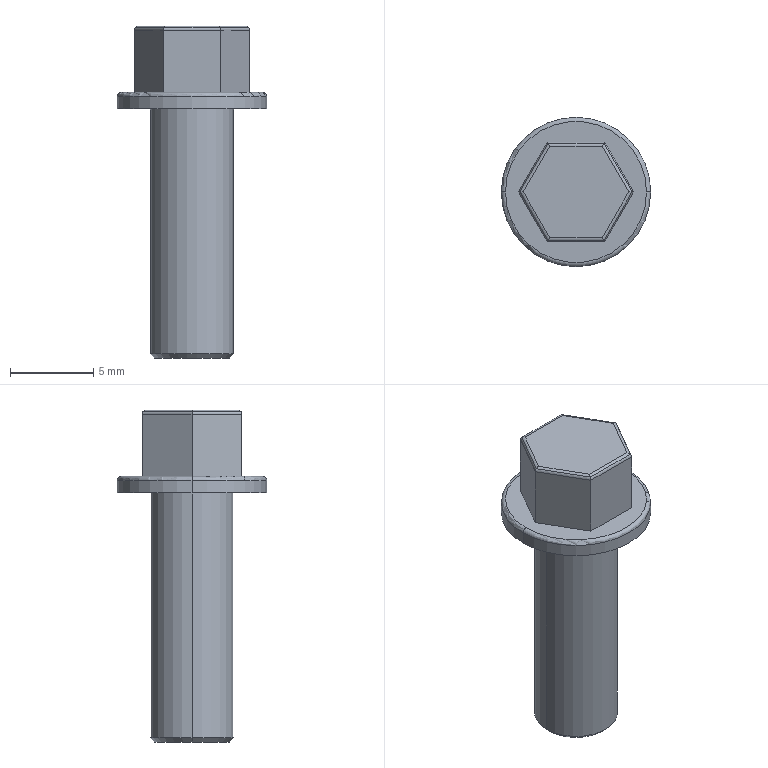Part | SolidWorks | features BaseBody 1 | 1 solid | 30 faces | box 9 x 9 x 20 mm | volume 481.727 mm3 | cylinder 16 | plane 10 | torus 2 | cone 2 | commonest cylinder face diameters 0.5 x12 5 x2 9 x2
STEP:
#1=CARTESIAN_POINT('',(-1.69,2.927,4.927));
#2=VERTEX_POINT('',#1);
#3=CARTESIAN_POINT('',(-1.732,3.,4.75));
#4=VERTEX_POINT('',#3);
#5=CARTESIAN_POINT('',(-1.69,2.927,4.927));
#6=CARTESIAN_POINT('',(-1.717,2.974,4.879));
#7=CARTESIAN_POINT('',(-1.732,3.,4.817));
#8=CARTESIAN_POINT('',(-1.732,3.,4.75));
#9=(BOUNDED_CURVE()B_SPLINE_CURVE(3,(#5,#6,#7,#8),.UNSPECIFIED.,.F.,.F.)B_SPLINE_CURVE_WITH_KNOTS((4,4),(5.498,6.283),.UNSPECIFIED.)CURVE()GEOMETRIC_REPRESENTATION_ITEM()RATIONAL_B_SPLINE_CURVE((1.,0.9493,0.9493,1.))REPRESENTATION_ITEM(''));
#10=EDGE_CURVE('',#2,#4,#9,.T.);
#11=ORIENTED_EDGE('',*,*,#10,.F.);
#12=CARTESIAN_POINT('',(1.69,2.927,4.927));
#13=VERTEX_POINT('',#12);
#14=CARTESIAN_POINT('',(0.866,2.927,4.927));
#15=DIRECTION('',(1.,0.,0.));
#16=VECTOR('',#15,1000.);
#17=LINE('',#14,#16);
#18=EDGE_CURVE('',#2,#13,#17,.T.);
#19=ORIENTED_EDGE('',*,*,#18,.T.);
#20=CARTESIAN_POINT('',(1.732,3.,4.75));
#21=VERTEX_POINT('',#20);
#22=CARTESIAN_POINT('',(1.69,2.927,4.927));
#23=CARTESIAN_POINT('',(1.717,2.974,4.879));
#24=CARTESIAN_POINT('',(1.732,3.,4.817));
#25=CARTESIAN_POINT('',(1.732,3.,4.75));
#26=(BOUNDED_CURVE()B_SPLINE_CURVE(3,(#22,#23,#24,#25),.UNSPECIFIED.,.F.,.F.)B_SPLINE_CURVE_WITH_KNOTS((4,4),(5.498,6.283),.UNSPECIFIED.)CURVE()GEOMETRIC_REPRESENTATION_ITEM()RATIONAL_B_SPLINE_CURVE((1.,0.9493,0.9493,1.))REPRESENTATION_ITEM(''));
#27=EDGE_CURVE('',#13,#21,#26,.T.);
#28=ORIENTED_EDGE('',*,*,#27,.T.);
#29=CARTESIAN_POINT('',(0.866,3.,4.75));
#30=DIRECTION('',(-1.,0.,0.));
#31=VECTOR('',#30,1000.);
#32=LINE('',#29,#31);
#33=EDGE_CURVE('',#21,#4,#32,.T.);
#34=ORIENTED_EDGE('',*,*,#33,.T.);
#35=EDGE_LOOP('',(#11,#19,#28,#34));
#36=FACE_OUTER_BOUND('',#35,.T.);
#37=CARTESIAN_POINT('',(0.866,2.75,4.75));
#38=DIRECTION('',(1.,0.,0.));
#39=DIRECTION('',(0.,0.7071,0.7071));
#40=AXIS2_PLACEMENT_3D('',#37,#38,#39);
#41=CYLINDRICAL_SURFACE('',#40,0.25);
#42=ADVANCED_FACE('',(#36),#41,.T.);
#43=ORIENTED_EDGE('',*,*,#27,.F.);
#44=CARTESIAN_POINT('',(3.38,0.,4.927));
#45=VERTEX_POINT('',#44);
#46=CARTESIAN_POINT('',(2.968,0.7134,4.927));
#47=DIRECTION('',(0.5,-0.866,0.));
#48=VECTOR('',#47,1000.);
#49=LINE('',#46,#48);
#50=EDGE_CURVE('',#13,#45,#49,.T.);
#51=ORIENTED_EDGE('',*,*,#50,.T.);
#52=CARTESIAN_POINT('',(3.464,0.,4.75));
#53=VERTEX_POINT('',#52);
#54=CARTESIAN_POINT('',(3.38,0.,4.927));
#55=CARTESIAN_POINT('',(3.434,0.,4.879));
#56=CARTESIAN_POINT('',(3.464,0.,4.817));
#57=CARTESIAN_POINT('',(3.464,0.,4.75));
#58=(BOUNDED_CURVE()B_SPLINE_CURVE(3,(#54,#55,#56,#57),.UNSPECIFIED.,.F.,.F.)B_SPLINE_CURVE_WITH_KNOTS((4,4),(5.498,6.283),.UNSPECIFIED.)CURVE()GEOMETRIC_REPRESENTATION_ITEM()RATIONAL_B_SPLINE_CURVE((1.,0.9493,0.9493,1.))REPRESENTATION_ITEM(''));
#59=EDGE_CURVE('',#45,#53,#58,.T.);
#60=ORIENTED_EDGE('',*,*,#59,.T.);
#61=CARTESIAN_POINT('',(3.031,0.75,4.75));
#62=DIRECTION('',(-0.5,0.866,0.));
#63=VECTOR('',#62,1000.);
#64=LINE('',#61,#63);
#65=EDGE_CURVE('',#53,#21,#64,.T.);
#66=ORIENTED_EDGE('',*,*,#65,.T.);
#67=EDGE_LOOP('',(#43,#51,#60,#66));
#68=FACE_OUTER_BOUND('',#67,.T.);
#69=CARTESIAN_POINT('',(2.815,0.625,4.75));
#70=DIRECTION('',(0.5,-0.866,0.));
#71=DIRECTION('',(0.6124,0.3536,0.7071));
#72=AXIS2_PLACEMENT_3D('',#69,#70,#71);
#73=CYLINDRICAL_SURFACE('',#72,0.25);
#74=ADVANCED_FACE('',(#68),#73,.T.);
#75=ORIENTED_EDGE('',*,*,#59,.F.);
#76=CARTESIAN_POINT('',(1.69,-2.927,4.927));
#77=VERTEX_POINT('',#76);
#78=CARTESIAN_POINT('',(2.102,-2.213,4.927));
#79=DIRECTION('',(-0.5,-0.866,0.));
#80=VECTOR('',#79,1000.);
#81=LINE('',#78,#80);
#82=EDGE_CURVE('',#45,#77,#81,.T.);
#83=ORIENTED_EDGE('',*,*,#82,.T.);
#84=CARTESIAN_POINT('',(1.732,-3.,4.75));
#85=VERTEX_POINT('',#84);
#86=CARTESIAN_POINT('',(1.69,-2.927,4.927));
#87=CARTESIAN_POINT('',(1.717,-2.974,4.879));
#88=CARTESIAN_POINT('',(1.732,-3.,4.817));
#89=CARTESIAN_POINT('',(1.732,-3.,4.75));
#90=(BOUNDED_CURVE()B_SPLINE_CURVE(3,(#86,#87,#88,#89),.UNSPECIFIED.,.F.,.F.)B_SPLINE_CURVE_WITH_KNOTS((4,4),(5.498,6.283),.UNSPECIFIED.)CURVE()GEOMETRIC_REPRESENTATION_ITEM()RATIONAL_B_SPLINE_CURVE((1.,0.9493,0.9493,1.))REPRESENTATION_ITEM(''));
#91=EDGE_CURVE('',#77,#85,#90,.T.);
#92=ORIENTED_EDGE('',*,*,#91,.T.);
#93=CARTESIAN_POINT('',(2.165,-2.25,4.75));
#94=DIRECTION('',(0.5,0.866,0.));
#95=VECTOR('',#94,1000.);
#96=LINE('',#93,#95);
#97=EDGE_CURVE('',#85,#53,#96,.T.);
#98=ORIENTED_EDGE('',*,*,#97,.T.);
#99=EDGE_LOOP('',(#75,#83,#92,#98));
#100=FACE_OUTER_BOUND('',#99,.T.);
#101=CARTESIAN_POINT('',(1.949,-2.125,4.75));
#102=DIRECTION('',(-0.5,-0.866,0.));
#103=DIRECTION('',(0.6124,-0.3536,0.7071));
#104=AXIS2_PLACEMENT_3D('',#101,#102,#103);
#105=CYLINDRICAL_SURFACE('',#104,0.25);
#106=ADVANCED_FACE('',(#100),#105,.T.);
#107=ORIENTED_EDGE('',*,*,#91,.F.);
#108=CARTESIAN_POINT('',(-1.69,-2.927,4.927));
#109=VERTEX_POINT('',#108);
#110=CARTESIAN_POINT('',(-0.866,-2.927,4.927));
#111=DIRECTION('',(-1.,0.,0.));
#112=VECTOR('',#111,1000.);
#113=LINE('',#110,#112);
#114=EDGE_CURVE('',#77,#109,#113,.T.);
#115=ORIENTED_EDGE('',*,*,#114,.T.);
#116=CARTESIAN_POINT('',(-1.732,-3.,4.75));
#117=VERTEX_POINT('',#116);
#118=CARTESIAN_POINT('',(-1.69,-2.927,4.927));
#119=CARTESIAN_POINT('',(-1.717,-2.974,4.879));
#120=CARTESIAN_POINT('',(-1.732,-3.,4.817));
#121=CARTESIAN_POINT('',(-1.732,-3.,4.75));
#122=(BOUNDED_CURVE()B_SPLINE_CURVE(3,(#118,#119,#120,#121),.UNSPECIFIED.,.F.,.F.)B_SPLINE_CURVE_WITH_KNOTS((4,4),(5.498,6.283),.UNSPECIFIED.)CURVE()GEOMETRIC_REPRESENTATION_ITEM()RATIONAL_B_SPLINE_CURVE((1.,0.9493,0.9493,1.))REPRESENTATION_ITEM(''));
#123=EDGE_CURVE('',#109,#117,#122,.T.);
#124=ORIENTED_EDGE('',*,*,#123,.T.);
#125=CARTESIAN_POINT('',(-0.866,-3.,4.75));
#126=DIRECTION('',(1.,0.,0.));
#127=VECTOR('',#126,1000.);
#128=LINE('',#125,#127);
#129=EDGE_CURVE('',#117,#85,#128,.T.);
#130=ORIENTED_EDGE('',*,*,#129,.T.);
#131=EDGE_LOOP('',(#107,#115,#124,#130));
#132=FACE_OUTER_BOUND('',#131,.T.);
#133=CARTESIAN_POINT('',(-0.866,-2.75,4.75));
#134=DIRECTION('',(-1.,0.,0.));
#135=DIRECTION('',(0.,-0.7071,0.7071));
#136=AXIS2_PLACEMENT_3D('',#133,#134,#135);
#137=CYLINDRICAL_SURFACE('',#136,0.25);
#138=ADVANCED_FACE('',(#132),#137,.T.);
#139=ORIENTED_EDGE('',*,*,#123,.F.);
#140=CARTESIAN_POINT('',(-3.38,0.,4.927));
#141=VERTEX_POINT('',#140);
#142=CARTESIAN_POINT('',(-2.968,-0.7134,4.927));
#143=DIRECTION('',(-0.5,0.866,0.));
#144=VECTOR('',#143,1000.);
#145=LINE('',#142,#144);
#146=EDGE_CURVE('',#109,#141,#145,.T.);
#147=ORIENTED_EDGE('',*,*,#146,.T.);
#148=CARTESIAN_POINT('',(-3.464,0.,4.75));
#149=VERTEX_POINT('',#148);
#150=CARTESIAN_POINT('',(-3.38,0.,4.927));
#151=CARTESIAN_POINT('',(-3.434,0.,4.879));
#152=CARTESIAN_POINT('',(-3.464,0.,4.817));
#153=CARTESIAN_POINT('',(-3.464,0.,4.75));
#154=(BOUNDED_CURVE()B_SPLINE_CURVE(3,(#150,#151,#152,#153),.UNSPECIFIED.,.F.,.F.)B_SPLINE_CURVE_WITH_KNOTS((4,4),(5.498,6.283),.UNSPECIFIED.)CURVE()GEOMETRIC_REPRESENTATION_ITEM()RATIONAL_B_SPLINE_CURVE((1.,0.9493,0.9493,1.))REPRESENTATION_ITEM(''));
#155=EDGE_CURVE('',#141,#149,#154,.T.);
#156=ORIENTED_EDGE('',*,*,#155,.T.);
#157=CARTESIAN_POINT('',(-3.031,-0.75,4.75));
#158=DIRECTION('',(0.5,-0.866,0.));
#159=VECTOR('',#158,1000.);
#160=LINE('',#157,#159);
#161=EDGE_CURVE('',#149,#117,#160,.T.);
#162=ORIENTED_EDGE('',*,*,#161,.T.);
#163=EDGE_LOOP('',(#139,#147,#156,#162));
#164=FACE_OUTER_BOUND('',#163,.T.);
#165=CARTESIAN_POINT('',(-2.815,-0.625,4.75));
#166=DIRECTION('',(-0.5,0.866,0.));
#167=DIRECTION('',(-0.6124,-0.3536,0.7071));
#168=AXIS2_PLACEMENT_3D('',#165,#166,#167);
#169=CYLINDRICAL_SURFACE('',#168,0.25);
#170=ADVANCED_FACE('',(#164),#169,.T.);
#171=ORIENTED_EDGE('',*,*,#155,.F.);
#172=CARTESIAN_POINT('',(-2.102,2.213,4.927));
#173=DIRECTION('',(0.5,0.866,0.));
#174=VECTOR('',#173,1000.);
#175=LINE('',#172,#174);
#176=EDGE_CURVE('',#141,#2,#175,.T.);
#177=ORIENTED_EDGE('',*,*,#176,.T.);
#178=ORIENTED_EDGE('',*,*,#10,.T.);
#179=CARTESIAN_POINT('',(-2.165,2.25,4.75));
#180=DIRECTION('',(-0.5,-0.866,0.));
#181=VECTOR('',#180,1000.);
#182=LINE('',#179,#181);
#183=EDGE_CURVE('',#4,#149,#182,.T.);
#184=ORIENTED_EDGE('',*,*,#183,.T.);
#185=EDGE_LOOP('',(#171,#177,#178,#184));
#186=FACE_OUTER_BOUND('',#185,.T.);
#187=CARTESIAN_POINT('',(-1.949,2.125,4.75));
#188=DIRECTION('',(0.5,0.866,0.));
#189=DIRECTION('',(-0.6124,0.3536,0.7071));
#190=AXIS2_PLACEMENT_3D('',#187,#188,#189);
#191=CYLINDRICAL_SURFACE('',#190,0.25);
#192=ADVANCED_FACE('',(#186),#191,.T.);
#193=CARTESIAN_POINT('',(4.5,0.,0.75));
#194=VERTEX_POINT('',#193);
#195=CARTESIAN_POINT('',(-4.5,0.,0.75));
#196=VERTEX_POINT('',#195);
#197=CARTESIAN_POINT('',(0.,0.,0.75));
#198=DIRECTION('',(0.,0.,1.));
#199=DIRECTION('',(-1.,0.,0.));
#200=AXIS2_PLACEMENT_3D('',#197,#198,#199);
#201=CIRCLE('',#200,4.5);
#202=EDGE_CURVE('',#194,#196,#201,.T.);
#203=ORIENTED_EDGE('',*,*,#202,.T.);
#204=CARTESIAN_POINT('',(-4.25,0.,1.));
#205=VERTEX_POINT('',#204);
#206=CARTESIAN_POINT('',(-4.25,0.,0.75));
#207=DIRECTION('',(0.,1.,0.));
#208=DIRECTION('',(-1.,0.,0.));
#209=AXIS2_PLACEMENT_3D('',#206,#207,#208);
#210=CIRCLE('',#209,0.25);
#211=EDGE_CURVE('',#196,#205,#210,.T.);
#212=ORIENTED_EDGE('',*,*,#211,.T.);
#213=CARTESIAN_POINT('',(4.25,0.,1.));
#214=VERTEX_POINT('',#213);
#215=CARTESIAN_POINT('',(0.,0.,1.));
#216=DIRECTION('',(0.,0.,-1.));
#217=DIRECTION('',(-1.,0.,0.));
#218=AXIS2_PLACEMENT_3D('',#215,#216,#217);
#219=CIRCLE('',#218,4.25);
#220=EDGE_CURVE('',#205,#214,#219,.T.);
#221=ORIENTED_EDGE('',*,*,#220,.T.);
#222=CARTESIAN_POINT('',(4.25,0.,0.75));
#223=DIRECTION('',(0.,-1.,0.));
#224=DIRECTION('',(0.,0.,-1.));
#225=AXIS2_PLACEMENT_3D('',#222,#223,#224);
#226=CIRCLE('',#225,0.25);
#227=EDGE_CURVE('',#194,#214,#226,.T.);
#228=ORIENTED_EDGE('',*,*,#227,.F.);
#229=EDGE_LOOP('',(#203,#212,#221,#228));
#230=FACE_OUTER_BOUND('',#229,.T.);
#231=CARTESIAN_POINT('',(0.,0.,0.75));
#232=DIRECTION('',(0.,0.,1.));
#233=DIRECTION('',(1.,0.,0.));
#234=AXIS2_PLACEMENT_3D('',#231,#232,#233);
#235=TOROIDAL_SURFACE('',#234,4.25,0.25);
#236=ADVANCED_FACE('',(#230),#235,.T.);
#237=ORIENTED_EDGE('',*,*,#202,.F.);
#238=CARTESIAN_POINT('',(4.5,0.,0.));
#239=VERTEX_POINT('',#238);
#240=CARTESIAN_POINT('',(4.5,0.,0.));
#241=DIRECTION('',(0.,0.,-1.));
#242=VECTOR('',#241,1000.);
#243=LINE('',#240,#242);
#244=EDGE_CURVE('',#194,#239,#243,.T.);
#245=ORIENTED_EDGE('',*,*,#244,.T.);
#246=CARTESIAN_POINT('',(-4.5,0.,0.));
#247=VERTEX_POINT('',#246);
#248=CARTESIAN_POINT('',(0.,0.,0.));
#249=DIRECTION('',(0.,0.,-1.));
#250=DIRECTION('',(-1.,0.,0.));
#251=AXIS2_PLACEMENT_3D('',#248,#249,#250);
#252=CIRCLE('',#251,4.5);
#253=EDGE_CURVE('',#247,#239,#252,.T.);
#254=ORIENTED_EDGE('',*,*,#253,.F.);
#255=CARTESIAN_POINT('',(-4.5,0.,0.));
#256=DIRECTION('',(0.,0.,-1.));
#257=VECTOR('',#256,1000.);
#258=LINE('',#255,#257);
#259=EDGE_CURVE('',#196,#247,#258,.T.);
#260=ORIENTED_EDGE('',*,*,#259,.F.);
#261=EDGE_LOOP('',(#237,#245,#254,#260));
#262=FACE_OUTER_BOUND('',#261,.T.);
#263=CARTESIAN_POINT('',(0.,0.,0.));
#264=DIRECTION('',(0.,0.,-1.));
#265=DIRECTION('',(-1.,0.,0.));
#266=AXIS2_PLACEMENT_3D('',#263,#264,#265);
#267=CYLINDRICAL_SURFACE('',#266,4.5);
#268=ADVANCED_FACE('',(#262),#267,.T.);
#269=CARTESIAN_POINT('',(2.25,0.,-15.));
#270=VERTEX_POINT('',#269);
#271=CARTESIAN_POINT('',(-2.25,0.,-15.));
#272=VERTEX_POINT('',#271);
#273=CARTESIAN_POINT('',(0.,0.,-15.));
#274=DIRECTION('',(0.,0.,1.));
#275=DIRECTION('',(1.,0.,0.));
#276=AXIS2_PLACEMENT_3D('',#273,#274,#275);
#277=CIRCLE('',#276,2.25);
#278=EDGE_CURVE('',#270,#272,#277,.T.);
#279=ORIENTED_EDGE('',*,*,#278,.T.);
#280=CARTESIAN_POINT('',(-2.5,0.,-14.75));
#281=VERTEX_POINT('',#280);
#282=CARTESIAN_POINT('',(-2.375,0.,-14.875));
#283=DIRECTION('',(-0.7071,0.,0.7071));
#284=VECTOR('',#283,1000.);
#285=LINE('',#282,#284);
#286=EDGE_CURVE('',#272,#281,#285,.T.);
#287=ORIENTED_EDGE('',*,*,#286,.T.);
#288=CARTESIAN_POINT('',(2.5,0.,-14.75));
#289=VERTEX_POINT('',#288);
#290=CARTESIAN_POINT('',(0.,0.,-14.75));
#291=DIRECTION('',(0.,0.,-1.));
#292=DIRECTION('',(1.,0.,0.));
#293=AXIS2_PLACEMENT_3D('',#290,#291,#292);
#294=CIRCLE('',#293,2.5);
#295=EDGE_CURVE('',#281,#289,#294,.T.);
#296=ORIENTED_EDGE('',*,*,#295,.T.);
#297=CARTESIAN_POINT('',(2.375,0.,-14.875));
#298=DIRECTION('',(0.7071,0.,0.7071));
#299=VECTOR('',#298,1000.);
#300=LINE('',#297,#299);
#301=EDGE_CURVE('',#270,#289,#300,.T.);
#302=ORIENTED_EDGE('',*,*,#301,.F.);
#303=EDGE_LOOP('',(#279,#287,#296,#302));
#304=FACE_OUTER_BOUND('',#303,.T.);
#305=CARTESIAN_POINT('',(0.,0.,-14.875));
#306=DIRECTION('',(0.,0.,1.));
#307=DIRECTION('',(1.,0.,0.));
#308=AXIS2_PLACEMENT_3D('',#305,#306,#307);
#309=CONICAL_SURFACE('',#308,2.375,0.7854);
#310=ADVANCED_FACE('',(#304),#309,.T.);
#311=ORIENTED_EDGE('',*,*,#295,.F.);
#312=CARTESIAN_POINT('',(-2.5,0.,0.));
#313=VERTEX_POINT('',#312);
#314=CARTESIAN_POINT('',(-2.5,0.,0.));
#315=DIRECTION('',(0.,0.,1.));
#316=VECTOR('',#315,1000.);
#317=LINE('',#314,#316);
#318=EDGE_CURVE('',#281,#313,#317,.T.);
#319=ORIENTED_EDGE('',*,*,#318,.T.);
#320=CARTESIAN_POINT('',(2.5,0.,0.));
#321=VERTEX_POINT('',#320);
#322=CARTESIAN_POINT('',(0.,0.,0.));
#323=DIRECTION('',(0.,0.,1.));
#324=DIRECTION('',(1.,0.,0.));
#325=AXIS2_PLACEMENT_3D('',#322,#323,#324);
#326=CIRCLE('',#325,2.5);
#327=EDGE_CURVE('',#321,#313,#326,.T.);
#328=ORIENTED_EDGE('',*,*,#327,.F.);
#329=CARTESIAN_POINT('',(2.5,0.,0.));
#330=DIRECTION('',(0.,0.,1.));
#331=VECTOR('',#330,1000.);
#332=LINE('',#329,#331);
#333=EDGE_CURVE('',#289,#321,#332,.T.);
#334=ORIENTED_EDGE('',*,*,#333,.F.);
#335=EDGE_LOOP('',(#311,#319,#328,#334));
#336=FACE_OUTER_BOUND('',#335,.T.);
#337=CARTESIAN_POINT('',(0.,0.,0.));
#338=DIRECTION('',(0.,0.,1.));
#339=DIRECTION('',(1.,0.,0.));
#340=AXIS2_PLACEMENT_3D('',#337,#338,#339);
#341=CYLINDRICAL_SURFACE('',#340,2.5);
#342=ADVANCED_FACE('',(#336),#341,.T.);
#343=ORIENTED_EDGE('',*,*,#161,.F.);
#344=CARTESIAN_POINT('',(-3.464,0.,1.));
#345=VERTEX_POINT('',#344);
#346=CARTESIAN_POINT('',(-3.464,0.,1.));
#347=DIRECTION('',(0.,0.,1.));
#348=VECTOR('',#347,1000.);
#349=LINE('',#346,#348);
#350=EDGE_CURVE('',#345,#149,#349,.T.);
#351=ORIENTED_EDGE('',*,*,#350,.F.);
#352=CARTESIAN_POINT('',(-1.732,-3.,1.));
#353=VERTEX_POINT('',#352);
#354=CARTESIAN_POINT('',(-3.031,-0.75,1.));
#355=DIRECTION('',(-0.5,0.866,0.));
#356=VECTOR('',#355,1000.);
#357=LINE('',#354,#356);
#358=EDGE_CURVE('',#353,#345,#357,.T.);
#359=ORIENTED_EDGE('',*,*,#358,.F.);
#360=CARTESIAN_POINT('',(-1.732,-3.,1.));
#361=DIRECTION('',(0.,0.,1.));
#362=VECTOR('',#361,1000.);
#363=LINE('',#360,#362);
#364=EDGE_CURVE('',#353,#117,#363,.T.);
#365=ORIENTED_EDGE('',*,*,#364,.T.);
#366=EDGE_LOOP('',(#343,#351,#359,#365));
#367=FACE_OUTER_BOUND('',#366,.T.);
#368=CARTESIAN_POINT('',(-3.464,0.,1.));
#369=DIRECTION('',(-0.866,-0.5,0.));
#370=DIRECTION('',(-0.5,0.866,0.));
#371=AXIS2_PLACEMENT_3D('',#368,#369,#370);
#372=PLANE('',#371);
#373=ADVANCED_FACE('',(#367),#372,.T.);
#374=ORIENTED_EDGE('',*,*,#183,.F.);
#375=CARTESIAN_POINT('',(-1.732,3.,1.));
#376=VERTEX_POINT('',#375);
#377=CARTESIAN_POINT('',(-1.732,3.,1.));
#378=DIRECTION('',(0.,0.,1.));
#379=VECTOR('',#378,1000.);
#380=LINE('',#377,#379);
#381=EDGE_CURVE('',#376,#4,#380,.T.);
#382=ORIENTED_EDGE('',*,*,#381,.F.);
#383=CARTESIAN_POINT('',(-2.165,2.25,1.));
#384=DIRECTION('',(0.5,0.866,0.));
#385=VECTOR('',#384,1000.);
#386=LINE('',#383,#385);
#387=EDGE_CURVE('',#345,#376,#386,.T.);
#388=ORIENTED_EDGE('',*,*,#387,.F.);
#389=ORIENTED_EDGE('',*,*,#350,.T.);
#390=EDGE_LOOP('',(#374,#382,#388,#389));
#391=FACE_OUTER_BOUND('',#390,.T.);
#392=CARTESIAN_POINT('',(-1.732,3.,1.));
#393=DIRECTION('',(-0.866,0.5,0.));
#394=DIRECTION('',(0.,0.,1.));
#395=AXIS2_PLACEMENT_3D('',#392,#393,#394);
#396=PLANE('',#395);
#397=ADVANCED_FACE('',(#391),#396,.T.);
#398=ORIENTED_EDGE('',*,*,#33,.F.);
#399=CARTESIAN_POINT('',(1.732,3.,1.));
#400=VERTEX_POINT('',#399);
#401=CARTESIAN_POINT('',(1.732,3.,1.));
#402=DIRECTION('',(0.,0.,1.));
#403=VECTOR('',#402,1000.);
#404=LINE('',#401,#403);
#405=EDGE_CURVE('',#400,#21,#404,.T.);
#406=ORIENTED_EDGE('',*,*,#405,.F.);
#407=CARTESIAN_POINT('',(0.866,3.,1.));
#408=DIRECTION('',(1.,0.,0.));
#409=VECTOR('',#408,1000.);
#410=LINE('',#407,#409);
#411=EDGE_CURVE('',#376,#400,#410,.T.);
#412=ORIENTED_EDGE('',*,*,#411,.F.);
#413=ORIENTED_EDGE('',*,*,#381,.T.);
#414=EDGE_LOOP('',(#398,#406,#412,#413));
#415=FACE_OUTER_BOUND('',#414,.T.);
#416=CARTESIAN_POINT('',(1.732,3.,1.));
#417=DIRECTION('',(0.,1.,0.));
#418=DIRECTION('',(1.,0.,0.));
#419=AXIS2_PLACEMENT_3D('',#416,#417,#418);
#420=PLANE('',#419);
#421=ADVANCED_FACE('',(#415),#420,.T.);
#422=CARTESIAN_POINT('',(-1.588,2.75,5.));
#423=VERTEX_POINT('',#422);
#424=CARTESIAN_POINT('',(1.588,2.75,5.));
#425=VERTEX_POINT('',#424);
#426=CARTESIAN_POINT('',(0.866,2.75,5.));
#427=DIRECTION('',(1.,0.,0.));
#428=VECTOR('',#427,1000.);
#429=LINE('',#426,#428);
#430=EDGE_CURVE('',#423,#425,#429,.T.);
#431=ORIENTED_EDGE('',*,*,#430,.F.);
#432=CARTESIAN_POINT('',(-3.175,0.,5.));
#433=VERTEX_POINT('',#432);
#434=CARTESIAN_POINT('',(-1.949,2.125,5.));
#435=DIRECTION('',(0.5,0.866,0.));
#436=VECTOR('',#435,1000.);
#437=LINE('',#434,#436);
#438=EDGE_CURVE('',#433,#423,#437,.T.);
#439=ORIENTED_EDGE('',*,*,#438,.F.);
#440=CARTESIAN_POINT('',(-1.588,-2.75,5.));
#441=VERTEX_POINT('',#440);
#442=CARTESIAN_POINT('',(-2.815,-0.625,5.));
#443=DIRECTION('',(-0.5,0.866,0.));
#444=VECTOR('',#443,1000.);
#445=LINE('',#442,#444);
#446=EDGE_CURVE('',#441,#433,#445,.T.);
#447=ORIENTED_EDGE('',*,*,#446,.F.);
#448=CARTESIAN_POINT('',(1.588,-2.75,5.));
#449=VERTEX_POINT('',#448);
#450=CARTESIAN_POINT('',(-0.866,-2.75,5.));
#451=DIRECTION('',(-1.,0.,0.));
#452=VECTOR('',#451,1000.);
#453=LINE('',#450,#452);
#454=EDGE_CURVE('',#449,#441,#453,.T.);
#455=ORIENTED_EDGE('',*,*,#454,.F.);
#456=CARTESIAN_POINT('',(3.175,0.,5.));
#457=VERTEX_POINT('',#456);
#458=CARTESIAN_POINT('',(1.949,-2.125,5.));
#459=DIRECTION('',(-0.5,-0.866,0.));
#460=VECTOR('',#459,1000.);
#461=LINE('',#458,#460);
#462=EDGE_CURVE('',#457,#449,#461,.T.);
#463=ORIENTED_EDGE('',*,*,#462,.F.);
#464=CARTESIAN_POINT('',(2.815,0.625,5.));
#465=DIRECTION('',(0.5,-0.866,0.));
#466=VECTOR('',#465,1000.);
#467=LINE('',#464,#466);
#468=EDGE_CURVE('',#425,#457,#467,.T.);
#469=ORIENTED_EDGE('',*,*,#468,.F.);
#470=EDGE_LOOP('',(#431,#439,#447,#455,#463,#469));
#471=FACE_OUTER_BOUND('',#470,.T.);
#472=CARTESIAN_POINT('',(0.,0.,5.));
#473=DIRECTION('',(0.,0.,1.));
#474=DIRECTION('',(1.,0.,0.));
#475=AXIS2_PLACEMENT_3D('',#472,#473,#474);
#476=PLANE('',#475);
#477=ADVANCED_FACE('',(#471),#476,.T.);
#478=ORIENTED_EDGE('',*,*,#358,.T.);
#479=ORIENTED_EDGE('',*,*,#387,.T.);
#480=ORIENTED_EDGE('',*,*,#411,.T.);
#481=CARTESIAN_POINT('',(3.464,0.,1.));
#482=VERTEX_POINT('',#481);
#483=CARTESIAN_POINT('',(3.031,0.75,1.));
#484=DIRECTION('',(0.5,-0.866,0.));
#485=VECTOR('',#484,1000.);
#486=LINE('',#483,#485);
#487=EDGE_CURVE('',#400,#482,#486,.T.);
#488=ORIENTED_EDGE('',*,*,#487,.T.);
#489=CARTESIAN_POINT('',(1.732,-3.,1.));
#490=VERTEX_POINT('',#489);
#491=CARTESIAN_POINT('',(2.165,-2.25,1.));
#492=DIRECTION('',(-0.5,-0.866,0.));
#493=VECTOR('',#492,1000.);
#494=LINE('',#491,#493);
#495=EDGE_CURVE('',#482,#490,#494,.T.);
#496=ORIENTED_EDGE('',*,*,#495,.T.);
#497=CARTESIAN_POINT('',(-0.866,-3.,1.));
#498=DIRECTION('',(-1.,0.,0.));
#499=VECTOR('',#498,1000.);
#500=LINE('',#497,#499);
#501=EDGE_CURVE('',#490,#353,#500,.T.);
#502=ORIENTED_EDGE('',*,*,#501,.T.);
#503=EDGE_LOOP('',(#478,#479,#480,#488,#496,#502));
#504=FACE_BOUND('',#503,.T.);
#505=CARTESIAN_POINT('',(0.,0.,1.));
#506=DIRECTION('',(0.,0.,-1.));
#507=DIRECTION('',(-1.,0.,0.));
#508=AXIS2_PLACEMENT_3D('',#505,#506,#507);
#509=CIRCLE('',#508,4.25);
#510=EDGE_CURVE('',#214,#205,#509,.T.);
#511=ORIENTED_EDGE('',*,*,#510,.F.);
#512=ORIENTED_EDGE('',*,*,#220,.F.);
#513=EDGE_LOOP('',(#511,#512));
#514=FACE_OUTER_BOUND('',#513,.T.);
#515=CARTESIAN_POINT('',(0.,0.,1.));
#516=DIRECTION('',(0.,0.,1.));
#517=DIRECTION('',(1.,0.,0.));
#518=AXIS2_PLACEMENT_3D('',#515,#516,#517);
#519=PLANE('',#518);
#520=ADVANCED_FACE('',(#504,#514),#519,.T.);
#521=ORIENTED_EDGE('',*,*,#278,.F.);
#522=CARTESIAN_POINT('',(0.,0.,-15.));
#523=DIRECTION('',(0.,0.,1.));
#524=DIRECTION('',(1.,0.,0.));
#525=AXIS2_PLACEMENT_3D('',#522,#523,#524);
#526=CIRCLE('',#525,2.25);
#527=EDGE_CURVE('',#272,#270,#526,.T.);
#528=ORIENTED_EDGE('',*,*,#527,.F.);
#529=EDGE_LOOP('',(#521,#528));
#530=FACE_OUTER_BOUND('',#529,.T.);
#531=CARTESIAN_POINT('',(0.,0.,-15.));
#532=DIRECTION('',(0.,0.,1.));
#533=DIRECTION('',(1.,0.,0.));
#534=AXIS2_PLACEMENT_3D('',#531,#532,#533);
#535=PLANE('',#534);
#536=ADVANCED_FACE('',(#530),#535,.F.);
#537=ORIENTED_EDGE('',*,*,#65,.F.);
#538=CARTESIAN_POINT('',(3.464,0.,1.));
#539=DIRECTION('',(0.,0.,1.));
#540=VECTOR('',#539,1000.);
#541=LINE('',#538,#540);
#542=EDGE_CURVE('',#482,#53,#541,.T.);
#543=ORIENTED_EDGE('',*,*,#542,.F.);
#544=ORIENTED_EDGE('',*,*,#487,.F.);
#545=ORIENTED_EDGE('',*,*,#405,.T.);
#546=EDGE_LOOP('',(#537,#543,#544,#545));
#547=FACE_OUTER_BOUND('',#546,.T.);
#548=CARTESIAN_POINT('',(3.464,0.,1.));
#549=DIRECTION('',(0.866,0.5,0.));
#550=DIRECTION('',(0.,0.,-1.));
#551=AXIS2_PLACEMENT_3D('',#548,#549,#550);
#552=PLANE('',#551);
#553=ADVANCED_FACE('',(#547),#552,.T.);
#554=ORIENTED_EDGE('',*,*,#97,.F.);
#555=CARTESIAN_POINT('',(1.732,-3.,1.));
#556=DIRECTION('',(0.,0.,1.));
#557=VECTOR('',#556,1000.);
#558=LINE('',#555,#557);
#559=EDGE_CURVE('',#490,#85,#558,.T.);
#560=ORIENTED_EDGE('',*,*,#559,.F.);
#561=ORIENTED_EDGE('',*,*,#495,.F.);
#562=ORIENTED_EDGE('',*,*,#542,.T.);
#563=EDGE_LOOP('',(#554,#560,#561,#562));
#564=FACE_OUTER_BOUND('',#563,.T.);
#565=CARTESIAN_POINT('',(1.732,-3.,1.));
#566=DIRECTION('',(0.866,-0.5,0.));
#567=DIRECTION('',(0.,0.,-1.));
#568=AXIS2_PLACEMENT_3D('',#565,#566,#567);
#569=PLANE('',#568);
#570=ADVANCED_FACE('',(#564),#569,.T.);
#571=ORIENTED_EDGE('',*,*,#129,.F.);
#572=ORIENTED_EDGE('',*,*,#364,.F.);
#573=ORIENTED_EDGE('',*,*,#501,.F.);
#574=ORIENTED_EDGE('',*,*,#559,.T.);
#575=EDGE_LOOP('',(#571,#572,#573,#574));
#576=FACE_OUTER_BOUND('',#575,.T.);
#577=CARTESIAN_POINT('',(-1.732,-3.,1.));
#578=DIRECTION('',(0.,-1.,0.));
#579=DIRECTION('',(-1.,0.,0.));
#580=AXIS2_PLACEMENT_3D('',#577,#578,#579);
#581=PLANE('',#580);
#582=ADVANCED_FACE('',(#576),#581,.T.);
#583=ORIENTED_EDGE('',*,*,#327,.T.);
#584=CARTESIAN_POINT('',(0.,0.,0.));
#585=DIRECTION('',(0.,0.,1.));
#586=DIRECTION('',(1.,0.,0.));
#587=AXIS2_PLACEMENT_3D('',#584,#585,#586);
#588=CIRCLE('',#587,2.5);
#589=EDGE_CURVE('',#313,#321,#588,.T.);
#590=ORIENTED_EDGE('',*,*,#589,.T.);
#591=EDGE_LOOP('',(#583,#590));
#592=FACE_BOUND('',#591,.T.);
#593=ORIENTED_EDGE('',*,*,#253,.T.);
#594=CARTESIAN_POINT('',(0.,0.,0.));
#595=DIRECTION('',(0.,0.,-1.));
#596=DIRECTION('',(-1.,0.,0.));
#597=AXIS2_PLACEMENT_3D('',#594,#595,#596);
#598=CIRCLE('',#597,4.5);
#599=EDGE_CURVE('',#239,#247,#598,.T.);
#600=ORIENTED_EDGE('',*,*,#599,.T.);
#601=EDGE_LOOP('',(#593,#600));
#602=FACE_OUTER_BOUND('',#601,.T.);
#603=CARTESIAN_POINT('',(0.,0.,0.));
#604=DIRECTION('',(0.,0.,1.));
#605=DIRECTION('',(1.,0.,0.));
#606=AXIS2_PLACEMENT_3D('',#603,#604,#605);
#607=PLANE('',#606);
#608=ADVANCED_FACE('',(#592,#602),#607,.F.);
#609=ORIENTED_EDGE('',*,*,#318,.F.);
#610=CARTESIAN_POINT('',(0.,0.,-14.75));
#611=DIRECTION('',(0.,0.,-1.));
#612=DIRECTION('',(1.,0.,0.));
#613=AXIS2_PLACEMENT_3D('',#610,#611,#612);
#614=CIRCLE('',#613,2.5);
#615=EDGE_CURVE('',#289,#281,#614,.T.);
#616=ORIENTED_EDGE('',*,*,#615,.F.);
#617=ORIENTED_EDGE('',*,*,#333,.T.);
#618=ORIENTED_EDGE('',*,*,#589,.F.);
#619=EDGE_LOOP('',(#609,#616,#617,#618));
#620=FACE_OUTER_BOUND('',#619,.T.);
#621=CARTESIAN_POINT('',(0.,0.,0.));
#622=DIRECTION('',(0.,0.,1.));
#623=DIRECTION('',(1.,0.,0.));
#624=AXIS2_PLACEMENT_3D('',#621,#622,#623);
#625=CYLINDRICAL_SURFACE('',#624,2.5);
#626=ADVANCED_FACE('',(#620),#625,.T.);
#627=ORIENTED_EDGE('',*,*,#286,.F.);
#628=ORIENTED_EDGE('',*,*,#527,.T.);
#629=ORIENTED_EDGE('',*,*,#301,.T.);
#630=ORIENTED_EDGE('',*,*,#615,.T.);
#631=EDGE_LOOP('',(#627,#628,#629,#630));
#632=FACE_OUTER_BOUND('',#631,.T.);
#633=CARTESIAN_POINT('',(0.,0.,-14.875));
#634=DIRECTION('',(0.,0.,1.));
#635=DIRECTION('',(1.,0.,0.));
#636=AXIS2_PLACEMENT_3D('',#633,#634,#635);
#637=CONICAL_SURFACE('',#636,2.375,0.7854);
#638=ADVANCED_FACE('',(#632),#637,.T.);
#639=ORIENTED_EDGE('',*,*,#244,.F.);
#640=CARTESIAN_POINT('',(0.,0.,0.75));
#641=DIRECTION('',(0.,0.,1.));
#642=DIRECTION('',(-1.,0.,0.));
#643=AXIS2_PLACEMENT_3D('',#640,#641,#642);
#644=CIRCLE('',#643,4.5);
#645=EDGE_CURVE('',#196,#194,#644,.T.);
#646=ORIENTED_EDGE('',*,*,#645,.F.);
#647=ORIENTED_EDGE('',*,*,#259,.T.);
#648=ORIENTED_EDGE('',*,*,#599,.F.);
#649=EDGE_LOOP('',(#639,#646,#647,#648));
#650=FACE_OUTER_BOUND('',#649,.T.);
#651=CARTESIAN_POINT('',(0.,0.,0.));
#652=DIRECTION('',(0.,0.,-1.));
#653=DIRECTION('',(-1.,0.,0.));
#654=AXIS2_PLACEMENT_3D('',#651,#652,#653);
#655=CYLINDRICAL_SURFACE('',#654,4.5);
#656=ADVANCED_FACE('',(#650),#655,.T.);
#657=ORIENTED_EDGE('',*,*,#211,.F.);
#658=ORIENTED_EDGE('',*,*,#645,.T.);
#659=ORIENTED_EDGE('',*,*,#227,.T.);
#660=ORIENTED_EDGE('',*,*,#510,.T.);
#661=EDGE_LOOP('',(#657,#658,#659,#660));
#662=FACE_OUTER_BOUND('',#661,.T.);
#663=CARTESIAN_POINT('',(0.,0.,0.75));
#664=DIRECTION('',(0.,0.,1.));
#665=DIRECTION('',(1.,0.,0.));
#666=AXIS2_PLACEMENT_3D('',#663,#664,#665);
#667=TOROIDAL_SURFACE('',#666,4.25,0.25);
#668=ADVANCED_FACE('',(#662),#667,.T.);
#669=ORIENTED_EDGE('',*,*,#176,.F.);
#670=CARTESIAN_POINT('',(-3.175,0.,5.));
#671=CARTESIAN_POINT('',(-3.253,0.,5.));
#672=CARTESIAN_POINT('',(-3.325,0.,4.974));
#673=CARTESIAN_POINT('',(-3.38,0.,4.927));
#674=(BOUNDED_CURVE()B_SPLINE_CURVE(3,(#670,#671,#672,#673),.UNSPECIFIED.,.F.,.F.)B_SPLINE_CURVE_WITH_KNOTS((4,4),(4.712,5.498),.UNSPECIFIED.)CURVE()GEOMETRIC_REPRESENTATION_ITEM()RATIONAL_B_SPLINE_CURVE((1.,0.9493,0.9493,1.))REPRESENTATION_ITEM(''));
#675=EDGE_CURVE('',#433,#141,#674,.T.);
#676=ORIENTED_EDGE('',*,*,#675,.F.);
#677=ORIENTED_EDGE('',*,*,#438,.T.);
#678=CARTESIAN_POINT('',(-1.588,2.75,5.));
#679=CARTESIAN_POINT('',(-1.627,2.817,5.));
#680=CARTESIAN_POINT('',(-1.662,2.879,4.974));
#681=CARTESIAN_POINT('',(-1.69,2.927,4.927));
#682=(BOUNDED_CURVE()B_SPLINE_CURVE(3,(#678,#679,#680,#681),.UNSPECIFIED.,.F.,.F.)B_SPLINE_CURVE_WITH_KNOTS((4,4),(4.712,5.498),.UNSPECIFIED.)CURVE()GEOMETRIC_REPRESENTATION_ITEM()RATIONAL_B_SPLINE_CURVE((1.,0.9493,0.9493,1.))REPRESENTATION_ITEM(''));
#683=EDGE_CURVE('',#423,#2,#682,.T.);
#684=ORIENTED_EDGE('',*,*,#683,.T.);
#685=EDGE_LOOP('',(#669,#676,#677,#684));
#686=FACE_OUTER_BOUND('',#685,.T.);
#687=CARTESIAN_POINT('',(-1.949,2.125,4.75));
#688=DIRECTION('',(0.5,0.866,0.));
#689=DIRECTION('',(-0.6124,0.3536,0.7071));
#690=AXIS2_PLACEMENT_3D('',#687,#688,#689);
#691=CYLINDRICAL_SURFACE('',#690,0.25);
#692=ADVANCED_FACE('',(#686),#691,.T.);
#693=ORIENTED_EDGE('',*,*,#146,.F.);
#694=CARTESIAN_POINT('',(-1.588,-2.75,5.));
#695=CARTESIAN_POINT('',(-1.627,-2.817,5.));
#696=CARTESIAN_POINT('',(-1.662,-2.879,4.974));
#697=CARTESIAN_POINT('',(-1.69,-2.927,4.927));
#698=(BOUNDED_CURVE()B_SPLINE_CURVE(3,(#694,#695,#696,#697),.UNSPECIFIED.,.F.,.F.)B_SPLINE_CURVE_WITH_KNOTS((4,4),(4.712,5.498),.UNSPECIFIED.)CURVE()GEOMETRIC_REPRESENTATION_ITEM()RATIONAL_B_SPLINE_CURVE((1.,0.9493,0.9493,1.))REPRESENTATION_ITEM(''));
#699=EDGE_CURVE('',#441,#109,#698,.T.);
#700=ORIENTED_EDGE('',*,*,#699,.F.);
#701=ORIENTED_EDGE('',*,*,#446,.T.);
#702=ORIENTED_EDGE('',*,*,#675,.T.);
#703=EDGE_LOOP('',(#693,#700,#701,#702));
#704=FACE_OUTER_BOUND('',#703,.T.);
#705=CARTESIAN_POINT('',(-2.815,-0.625,4.75));
#706=DIRECTION('',(-0.5,0.866,0.));
#707=DIRECTION('',(-0.6124,-0.3536,0.7071));
#708=AXIS2_PLACEMENT_3D('',#705,#706,#707);
#709=CYLINDRICAL_SURFACE('',#708,0.25);
#710=ADVANCED_FACE('',(#704),#709,.T.);
#711=ORIENTED_EDGE('',*,*,#114,.F.);
#712=CARTESIAN_POINT('',(1.588,-2.75,5.));
#713=CARTESIAN_POINT('',(1.627,-2.817,5.));
#714=CARTESIAN_POINT('',(1.662,-2.879,4.974));
#715=CARTESIAN_POINT('',(1.69,-2.927,4.927));
#716=(BOUNDED_CURVE()B_SPLINE_CURVE(3,(#712,#713,#714,#715),.UNSPECIFIED.,.F.,.F.)B_SPLINE_CURVE_WITH_KNOTS((4,4),(4.712,5.498),.UNSPECIFIED.)CURVE()GEOMETRIC_REPRESENTATION_ITEM()RATIONAL_B_SPLINE_CURVE((1.,0.9493,0.9493,1.))REPRESENTATION_ITEM(''));
#717=EDGE_CURVE('',#449,#77,#716,.T.);
#718=ORIENTED_EDGE('',*,*,#717,.F.);
#719=ORIENTED_EDGE('',*,*,#454,.T.);
#720=ORIENTED_EDGE('',*,*,#699,.T.);
#721=EDGE_LOOP('',(#711,#718,#719,#720));
#722=FACE_OUTER_BOUND('',#721,.T.);
#723=CARTESIAN_POINT('',(-0.866,-2.75,4.75));
#724=DIRECTION('',(-1.,0.,0.));
#725=DIRECTION('',(0.,-0.7071,0.7071));
#726=AXIS2_PLACEMENT_3D('',#723,#724,#725);
#727=CYLINDRICAL_SURFACE('',#726,0.25);
#728=ADVANCED_FACE('',(#722),#727,.T.);
#729=ORIENTED_EDGE('',*,*,#82,.F.);
#730=CARTESIAN_POINT('',(3.175,0.,5.));
#731=CARTESIAN_POINT('',(3.253,0.,5.));
#732=CARTESIAN_POINT('',(3.325,0.,4.974));
#733=CARTESIAN_POINT('',(3.38,0.,4.927));
#734=(BOUNDED_CURVE()B_SPLINE_CURVE(3,(#730,#731,#732,#733),.UNSPECIFIED.,.F.,.F.)B_SPLINE_CURVE_WITH_KNOTS((4,4),(4.712,5.498),.UNSPECIFIED.)CURVE()GEOMETRIC_REPRESENTATION_ITEM()RATIONAL_B_SPLINE_CURVE((1.,0.9493,0.9493,1.))REPRESENTATION_ITEM(''));
#735=EDGE_CURVE('',#457,#45,#734,.T.);
#736=ORIENTED_EDGE('',*,*,#735,.F.);
#737=ORIENTED_EDGE('',*,*,#462,.T.);
#738=ORIENTED_EDGE('',*,*,#717,.T.);
#739=EDGE_LOOP('',(#729,#736,#737,#738));
#740=FACE_OUTER_BOUND('',#739,.T.);
#741=CARTESIAN_POINT('',(1.949,-2.125,4.75));
#742=DIRECTION('',(-0.5,-0.866,0.));
#743=DIRECTION('',(0.6124,-0.3536,0.7071));
#744=AXIS2_PLACEMENT_3D('',#741,#742,#743);
#745=CYLINDRICAL_SURFACE('',#744,0.25);
#746=ADVANCED_FACE('',(#740),#745,.T.);
#747=ORIENTED_EDGE('',*,*,#50,.F.);
#748=CARTESIAN_POINT('',(1.588,2.75,5.));
#749=CARTESIAN_POINT('',(1.627,2.817,5.));
#750=CARTESIAN_POINT('',(1.662,2.879,4.974));
#751=CARTESIAN_POINT('',(1.69,2.927,4.927));
#752=(BOUNDED_CURVE()B_SPLINE_CURVE(3,(#748,#749,#750,#751),.UNSPECIFIED.,.F.,.F.)B_SPLINE_CURVE_WITH_KNOTS((4,4),(4.712,5.498),.UNSPECIFIED.)CURVE()GEOMETRIC_REPRESENTATION_ITEM()RATIONAL_B_SPLINE_CURVE((1.,0.9493,0.9493,1.))REPRESENTATION_ITEM(''));
#753=EDGE_CURVE('',#425,#13,#752,.T.);
#754=ORIENTED_EDGE('',*,*,#753,.F.);
#755=ORIENTED_EDGE('',*,*,#468,.T.);
#756=ORIENTED_EDGE('',*,*,#735,.T.);
#757=EDGE_LOOP('',(#747,#754,#755,#756));
#758=FACE_OUTER_BOUND('',#757,.T.);
#759=CARTESIAN_POINT('',(2.815,0.625,4.75));
#760=DIRECTION('',(0.5,-0.866,0.));
#761=DIRECTION('',(0.6124,0.3536,0.7071));
#762=AXIS2_PLACEMENT_3D('',#759,#760,#761);
#763=CYLINDRICAL_SURFACE('',#762,0.25);
#764=ADVANCED_FACE('',(#758),#763,.T.);
#765=ORIENTED_EDGE('',*,*,#18,.F.);
#766=ORIENTED_EDGE('',*,*,#683,.F.);
#767=ORIENTED_EDGE('',*,*,#430,.T.);
#768=ORIENTED_EDGE('',*,*,#753,.T.);
#769=EDGE_LOOP('',(#765,#766,#767,#768));
#770=FACE_OUTER_BOUND('',#769,.T.);
#771=CARTESIAN_POINT('',(0.866,2.75,4.75));
#772=DIRECTION('',(1.,0.,0.));
#773=DIRECTION('',(0.,0.7071,0.7071));
#774=AXIS2_PLACEMENT_3D('',#771,#772,#773);
#775=CYLINDRICAL_SURFACE('',#774,0.25);
#776=ADVANCED_FACE('',(#770),#775,.T.);
#777=CLOSED_SHELL('',(#42,#74,#106,#138,#170,#192,#236,#268,#310,#342,#373,#397,#421,#477,#520,#536,#553,#570,#582,#608,#626,#638,#656,#668,#692,#710,#728,#746,#764,#776));
#778=MANIFOLD_SOLID_BREP('',#777);
#779=CARTESIAN_POINT('',(0.,0.,0.));
#780=DIRECTION('',(0.,0.,1.));
#781=DIRECTION('',(1.,0.,0.));
#782=AXIS2_PLACEMENT_3D('',#779,#780,#781);
#783=(LENGTH_UNIT()NAMED_UNIT(*)SI_UNIT(.MILLI.,.METRE.));
#784=UNCERTAINTY_MEASURE_WITH_UNIT(LENGTH_MEASURE(0.00001),#783,'','');
#785=(NAMED_UNIT(*)PLANE_ANGLE_UNIT()SI_UNIT($,.RADIAN.));
#786=(NAMED_UNIT(*)SI_UNIT($,.STERADIAN.)SOLID_ANGLE_UNIT());
#787=(GEOMETRIC_REPRESENTATION_CONTEXT(3)GLOBAL_UNCERTAINTY_ASSIGNED_CONTEXT((#784))GLOBAL_UNIT_ASSIGNED_CONTEXT((#783,#785,#786))REPRESENTATION_CONTEXT('',''));
#788=ADVANCED_BREP_SHAPE_REPRESENTATION('',(#778,#782),#787);